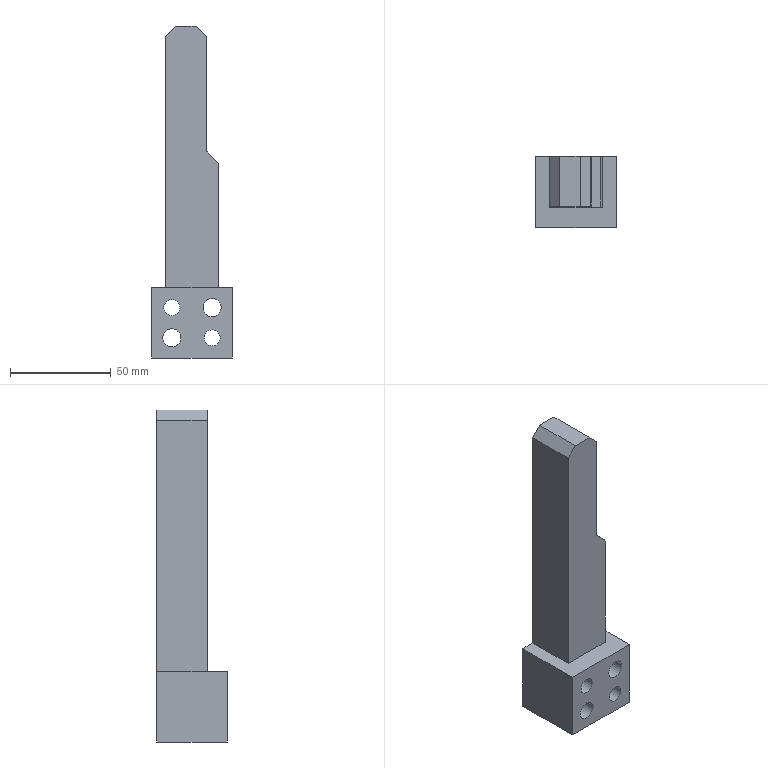Part | STEP file | 车灯-后视镜_id230_x_t | 1 solid | 24 faces | box 40 x 35 x 165 mm | volume 113527 mm3 | plane 16 | cylinder 8 | commonest cylinder face diameters 4 x2 8 x2 9 x2 14 x2
STEP:
#1=CARTESIAN_POINT('',(-100.914,285.,-263.086));
#2=VERTEX_POINT('',#1);
#3=CARTESIAN_POINT('',(-96.086,285.,-267.914));
#4=VERTEX_POINT('',#3);
#5=CARTESIAN_POINT('',(-53.5,285.,-310.5));
#6=DIRECTION('',(0.7071,0.,-0.7071));
#7=VECTOR('',#6,1.);
#8=LINE('',#5,#7);
#9=EDGE_CURVE('',#2,#4,#8,.T.);
#10=ORIENTED_EDGE('',*,*,#9,.T.);
#11=CARTESIAN_POINT('',(-96.086,310.,-267.914));
#12=VERTEX_POINT('',#11);
#13=CARTESIAN_POINT('',(-96.086,310.,-267.914));
#14=DIRECTION('',(0.,1.,0.));
#15=VECTOR('',#14,1.);
#16=LINE('',#13,#15);
#17=EDGE_CURVE('',#4,#12,#16,.T.);
#18=ORIENTED_EDGE('',*,*,#17,.T.);
#19=CARTESIAN_POINT('',(-100.914,310.,-263.086));
#20=VERTEX_POINT('',#19);
#21=CARTESIAN_POINT('',(-53.5,310.,-310.5));
#22=DIRECTION('',(-0.7071,0.,0.7071));
#23=VECTOR('',#22,1.);
#24=LINE('',#21,#23);
#25=EDGE_CURVE('',#12,#20,#24,.T.);
#26=ORIENTED_EDGE('',*,*,#25,.T.);
#27=CARTESIAN_POINT('',(-100.914,285.,-263.086));
#28=DIRECTION('',(0.,-1.,0.));
#29=VECTOR('',#28,1.);
#30=LINE('',#27,#29);
#31=EDGE_CURVE('',#20,#2,#30,.T.);
#32=ORIENTED_EDGE('',*,*,#31,.T.);
#33=EDGE_LOOP('',(#10,#18,#26,#32));
#34=FACE_OUTER_BOUND('',#33,.T.);
#35=CARTESIAN_POINT('',(-95.5,285.,-268.5));
#36=DIRECTION('',(0.7071,0.,0.7071));
#37=DIRECTION('',(-0.7071,0.,0.7071));
#38=AXIS2_PLACEMENT_3D('',#35,#36,#37);
#39=PLANE('',#38);
#40=ADVANCED_FACE('',(#34),#39,.T.);
#41=CARTESIAN_POINT('',(-121.5,285.,-330.5));
#42=VERTEX_POINT('',#41);
#43=CARTESIAN_POINT('',(-121.5,285.,-205.5));
#44=VERTEX_POINT('',#43);
#45=CARTESIAN_POINT('',(-121.5,285.,-365.5));
#46=DIRECTION('',(0.,0.,1.));
#47=VECTOR('',#46,1.);
#48=LINE('',#45,#47);
#49=EDGE_CURVE('',#42,#44,#48,.T.);
#50=ORIENTED_EDGE('',*,*,#49,.T.);
#51=CARTESIAN_POINT('',(-121.5,310.,-205.5));
#52=VERTEX_POINT('',#51);
#53=CARTESIAN_POINT('',(-121.5,310.,-205.5));
#54=DIRECTION('',(0.,1.,0.));
#55=VECTOR('',#54,1.);
#56=LINE('',#53,#55);
#57=EDGE_CURVE('',#44,#52,#56,.T.);
#58=ORIENTED_EDGE('',*,*,#57,.T.);
#59=CARTESIAN_POINT('',(-121.5,310.,-330.5));
#60=VERTEX_POINT('',#59);
#61=CARTESIAN_POINT('',(-121.5,310.,-365.5));
#62=DIRECTION('',(0.,0.,1.));
#63=VECTOR('',#62,1.);
#64=LINE('',#61,#63);
#65=EDGE_CURVE('',#60,#52,#64,.T.);
#66=ORIENTED_EDGE('',*,*,#65,.F.);
#67=CARTESIAN_POINT('',(-121.5,292.5,-330.5));
#68=DIRECTION('',(0.,-1.,0.));
#69=VECTOR('',#68,1.);
#70=LINE('',#67,#69);
#71=EDGE_CURVE('',#60,#42,#70,.T.);
#72=ORIENTED_EDGE('',*,*,#71,.T.);
#73=EDGE_LOOP('',(#50,#58,#66,#72));
#74=FACE_OUTER_BOUND('',#73,.T.);
#75=CARTESIAN_POINT('',(-121.5,292.5,-365.5));
#76=DIRECTION('',(-1.,0.,0.));
#77=DIRECTION('',(0.,0.,-1.));
#78=AXIS2_PLACEMENT_3D('',#75,#76,#77);
#79=PLANE('',#78);
#80=ADVANCED_FACE('',(#74),#79,.T.);
#81=CARTESIAN_POINT('',(-95.5,285.,-330.5));
#82=VERTEX_POINT('',#81);
#83=CARTESIAN_POINT('',(-95.5,285.,-269.328));
#84=VERTEX_POINT('',#83);
#85=CARTESIAN_POINT('',(-95.5,285.,-365.5));
#86=DIRECTION('',(0.,0.,1.));
#87=VECTOR('',#86,1.);
#88=LINE('',#85,#87);
#89=EDGE_CURVE('',#82,#84,#88,.T.);
#90=ORIENTED_EDGE('',*,*,#89,.T.);
#91=CARTESIAN_POINT('',(-97.5,285.,-269.328));
#92=DIRECTION('',(0.,-1.,0.));
#93=DIRECTION('',(0.,0.,1.));
#94=AXIS2_PLACEMENT_3D('',#91,#92,#93);
#95=CIRCLE('',#94,2.);
#96=EDGE_CURVE('',#84,#4,#95,.T.);
#97=ORIENTED_EDGE('',*,*,#96,.T.);
#98=ORIENTED_EDGE('',*,*,#9,.F.);
#99=CARTESIAN_POINT('',(-101.5,285.,-261.672));
#100=VERTEX_POINT('',#99);
#101=CARTESIAN_POINT('',(-99.5,285.,-261.672));
#102=DIRECTION('',(0.,1.,0.));
#103=DIRECTION('',(0.,0.,1.));
#104=AXIS2_PLACEMENT_3D('',#101,#102,#103);
#105=CIRCLE('',#104,2.);
#106=EDGE_CURVE('',#2,#100,#105,.T.);
#107=ORIENTED_EDGE('',*,*,#106,.T.);
#108=CARTESIAN_POINT('',(-101.5,285.,-205.5));
#109=VERTEX_POINT('',#108);
#110=CARTESIAN_POINT('',(-101.5,285.,-365.5));
#111=DIRECTION('',(0.,0.,1.));
#112=VECTOR('',#111,1.);
#113=LINE('',#110,#112);
#114=EDGE_CURVE('',#100,#109,#113,.T.);
#115=ORIENTED_EDGE('',*,*,#114,.T.);
#116=CARTESIAN_POINT('',(-106.5,285.,-200.5));
#117=VERTEX_POINT('',#116);
#118=CARTESIAN_POINT('',(-25.,285.,-282.));
#119=DIRECTION('',(-0.7071,0.,0.7071));
#120=VECTOR('',#119,1.);
#121=LINE('',#118,#120);
#122=EDGE_CURVE('',#109,#117,#121,.T.);
#123=ORIENTED_EDGE('',*,*,#122,.T.);
#124=CARTESIAN_POINT('',(-116.5,285.,-200.5));
#125=VERTEX_POINT('',#124);
#126=CARTESIAN_POINT('',(-108.5,285.,-200.5));
#127=DIRECTION('',(1.,0.,0.));
#128=VECTOR('',#127,1.);
#129=LINE('',#126,#128);
#130=EDGE_CURVE('',#125,#117,#129,.T.);
#131=ORIENTED_EDGE('',*,*,#130,.F.);
#132=CARTESIAN_POINT('',(-195.,285.,-279.));
#133=DIRECTION('',(-0.7071,0.,-0.7071));
#134=VECTOR('',#133,1.);
#135=LINE('',#132,#134);
#136=EDGE_CURVE('',#125,#44,#135,.T.);
#137=ORIENTED_EDGE('',*,*,#136,.T.);
#138=ORIENTED_EDGE('',*,*,#49,.F.);
#139=CARTESIAN_POINT('',(-108.5,285.,-330.5));
#140=DIRECTION('',(1.,0.,0.));
#141=VECTOR('',#140,1.);
#142=LINE('',#139,#141);
#143=EDGE_CURVE('',#42,#82,#142,.T.);
#144=ORIENTED_EDGE('',*,*,#143,.T.);
#145=EDGE_LOOP('',(#90,#97,#98,#107,#115,#123,#131,#137,#138,#144));
#146=FACE_OUTER_BOUND('',#145,.T.);
#147=CARTESIAN_POINT('',(-108.5,285.,-365.5));
#148=DIRECTION('',(0.,-1.,0.));
#149=DIRECTION('',(0.,0.,1.));
#150=AXIS2_PLACEMENT_3D('',#147,#148,#149);
#151=PLANE('',#150);
#152=ADVANCED_FACE('',(#146),#151,.T.);
#153=CARTESIAN_POINT('',(-95.5,310.,-330.5));
#154=VERTEX_POINT('',#153);
#155=CARTESIAN_POINT('',(-95.5,310.,-269.328));
#156=VERTEX_POINT('',#155);
#157=CARTESIAN_POINT('',(-95.5,310.,-365.5));
#158=DIRECTION('',(0.,0.,1.));
#159=VECTOR('',#158,1.);
#160=LINE('',#157,#159);
#161=EDGE_CURVE('',#154,#156,#160,.T.);
#162=ORIENTED_EDGE('',*,*,#161,.T.);
#163=CARTESIAN_POINT('',(-95.5,285.,-269.328));
#164=DIRECTION('',(0.,-1.,0.));
#165=VECTOR('',#164,1.);
#166=LINE('',#163,#165);
#167=EDGE_CURVE('',#156,#84,#166,.T.);
#168=ORIENTED_EDGE('',*,*,#167,.T.);
#169=ORIENTED_EDGE('',*,*,#89,.F.);
#170=CARTESIAN_POINT('',(-95.5,292.5,-330.5));
#171=DIRECTION('',(0.,1.,0.));
#172=VECTOR('',#171,1.);
#173=LINE('',#170,#172);
#174=EDGE_CURVE('',#82,#154,#173,.T.);
#175=ORIENTED_EDGE('',*,*,#174,.T.);
#176=EDGE_LOOP('',(#162,#168,#169,#175));
#177=FACE_OUTER_BOUND('',#176,.T.);
#178=CARTESIAN_POINT('',(-95.5,292.5,-365.5));
#179=DIRECTION('',(1.,0.,0.));
#180=DIRECTION('',(0.,0.,1.));
#181=AXIS2_PLACEMENT_3D('',#178,#179,#180);
#182=PLANE('',#181);
#183=ADVANCED_FACE('',(#177),#182,.T.);
#184=CARTESIAN_POINT('',(-111.5,310.,-355.5));
#185=VERTEX_POINT('',#184);
#186=CARTESIAN_POINT('',(-118.5,310.,-355.5));
#187=DIRECTION('',(0.,-1.,0.));
#188=DIRECTION('',(1.,0.,0.));
#189=AXIS2_PLACEMENT_3D('',#186,#187,#188);
#190=CIRCLE('',#189,7.);
#191=EDGE_CURVE('',#185,#185,#190,.T.);
#192=ORIENTED_EDGE('',*,*,#191,.T.);
#193=EDGE_LOOP('',(#192));
#194=FACE_BOUND('',#193,.T.);
#195=CARTESIAN_POINT('',(-91.5,310.,-340.5));
#196=VERTEX_POINT('',#195);
#197=CARTESIAN_POINT('',(-98.5,310.,-340.5));
#198=DIRECTION('',(0.,-1.,0.));
#199=DIRECTION('',(1.,0.,0.));
#200=AXIS2_PLACEMENT_3D('',#197,#198,#199);
#201=CIRCLE('',#200,7.);
#202=EDGE_CURVE('',#196,#196,#201,.T.);
#203=ORIENTED_EDGE('',*,*,#202,.T.);
#204=EDGE_LOOP('',(#203));
#205=FACE_BOUND('',#204,.T.);
#206=ORIENTED_EDGE('',*,*,#25,.F.);
#207=CARTESIAN_POINT('',(-97.5,310.,-269.328));
#208=DIRECTION('',(0.,1.,0.));
#209=DIRECTION('',(0.,0.,-1.));
#210=AXIS2_PLACEMENT_3D('',#207,#208,#209);
#211=CIRCLE('',#210,2.);
#212=EDGE_CURVE('',#12,#156,#211,.T.);
#213=ORIENTED_EDGE('',*,*,#212,.T.);
#214=ORIENTED_EDGE('',*,*,#161,.F.);
#215=CARTESIAN_POINT('',(-88.5,310.,-330.5));
#216=VERTEX_POINT('',#215);
#217=CARTESIAN_POINT('',(-108.5,310.,-330.5));
#218=DIRECTION('',(-1.,0.,0.));
#219=VECTOR('',#218,1.);
#220=LINE('',#217,#219);
#221=EDGE_CURVE('',#216,#154,#220,.T.);
#222=ORIENTED_EDGE('',*,*,#221,.F.);
#223=CARTESIAN_POINT('',(-88.5,310.,-365.5));
#224=VERTEX_POINT('',#223);
#225=CARTESIAN_POINT('',(-88.5,310.,-365.5));
#226=DIRECTION('',(0.,0.,1.));
#227=VECTOR('',#226,1.);
#228=LINE('',#225,#227);
#229=EDGE_CURVE('',#224,#216,#228,.T.);
#230=ORIENTED_EDGE('',*,*,#229,.F.);
#231=CARTESIAN_POINT('',(-128.5,310.,-365.5));
#232=VERTEX_POINT('',#231);
#233=CARTESIAN_POINT('',(-108.5,310.,-365.5));
#234=DIRECTION('',(-1.,0.,0.));
#235=VECTOR('',#234,1.);
#236=LINE('',#233,#235);
#237=EDGE_CURVE('',#224,#232,#236,.T.);
#238=ORIENTED_EDGE('',*,*,#237,.T.);
#239=CARTESIAN_POINT('',(-128.5,310.,-330.5));
#240=VERTEX_POINT('',#239);
#241=CARTESIAN_POINT('',(-128.5,310.,-365.5));
#242=DIRECTION('',(0.,0.,1.));
#243=VECTOR('',#242,1.);
#244=LINE('',#241,#243);
#245=EDGE_CURVE('',#232,#240,#244,.T.);
#246=ORIENTED_EDGE('',*,*,#245,.T.);
#247=CARTESIAN_POINT('',(-108.5,310.,-330.5));
#248=DIRECTION('',(-1.,0.,0.));
#249=VECTOR('',#248,1.);
#250=LINE('',#247,#249);
#251=EDGE_CURVE('',#60,#240,#250,.T.);
#252=ORIENTED_EDGE('',*,*,#251,.F.);
#253=ORIENTED_EDGE('',*,*,#65,.T.);
#254=CARTESIAN_POINT('',(-116.5,310.,-200.5));
#255=VERTEX_POINT('',#254);
#256=CARTESIAN_POINT('',(-195.,310.,-279.));
#257=DIRECTION('',(0.7071,0.,0.7071));
#258=VECTOR('',#257,1.);
#259=LINE('',#256,#258);
#260=EDGE_CURVE('',#52,#255,#259,.T.);
#261=ORIENTED_EDGE('',*,*,#260,.T.);
#262=CARTESIAN_POINT('',(-106.5,310.,-200.5));
#263=VERTEX_POINT('',#262);
#264=CARTESIAN_POINT('',(-108.5,310.,-200.5));
#265=DIRECTION('',(-1.,0.,0.));
#266=VECTOR('',#265,1.);
#267=LINE('',#264,#266);
#268=EDGE_CURVE('',#263,#255,#267,.T.);
#269=ORIENTED_EDGE('',*,*,#268,.F.);
#270=CARTESIAN_POINT('',(-101.5,310.,-205.5));
#271=VERTEX_POINT('',#270);
#272=CARTESIAN_POINT('',(-25.,310.,-282.));
#273=DIRECTION('',(0.7071,0.,-0.7071));
#274=VECTOR('',#273,1.);
#275=LINE('',#272,#274);
#276=EDGE_CURVE('',#263,#271,#275,.T.);
#277=ORIENTED_EDGE('',*,*,#276,.T.);
#278=CARTESIAN_POINT('',(-101.5,310.,-261.672));
#279=VERTEX_POINT('',#278);
#280=CARTESIAN_POINT('',(-101.5,310.,-365.5));
#281=DIRECTION('',(0.,0.,1.));
#282=VECTOR('',#281,1.);
#283=LINE('',#280,#282);
#284=EDGE_CURVE('',#279,#271,#283,.T.);
#285=ORIENTED_EDGE('',*,*,#284,.F.);
#286=CARTESIAN_POINT('',(-99.5,310.,-261.672));
#287=DIRECTION('',(0.,-1.,0.));
#288=DIRECTION('',(0.,0.,-1.));
#289=AXIS2_PLACEMENT_3D('',#286,#287,#288);
#290=CIRCLE('',#289,2.);
#291=EDGE_CURVE('',#279,#20,#290,.T.);
#292=ORIENTED_EDGE('',*,*,#291,.T.);
#293=EDGE_LOOP('',(#206,#213,#214,#222,#230,#238,#246,#252,#253,#261,#269,#277,#285,#292));
#294=FACE_BOUND('',#293,.T.);
#295=CARTESIAN_POINT('',(-98.5,310.,-359.5));
#296=VERTEX_POINT('',#295);
#297=CARTESIAN_POINT('',(-98.5,310.,-355.5));
#298=DIRECTION('',(0.,-1.,0.));
#299=DIRECTION('',(0.,0.,-1.));
#300=AXIS2_PLACEMENT_3D('',#297,#298,#299);
#301=CIRCLE('',#300,4.);
#302=EDGE_CURVE('',#296,#296,#301,.T.);
#303=ORIENTED_EDGE('',*,*,#302,.T.);
#304=EDGE_LOOP('',(#303));
#305=FACE_BOUND('',#304,.T.);
#306=CARTESIAN_POINT('',(-118.5,310.,-344.5));
#307=VERTEX_POINT('',#306);
#308=CARTESIAN_POINT('',(-118.5,310.,-340.5));
#309=DIRECTION('',(0.,-1.,0.));
#310=DIRECTION('',(0.,0.,-1.));
#311=AXIS2_PLACEMENT_3D('',#308,#309,#310);
#312=CIRCLE('',#311,4.);
#313=EDGE_CURVE('',#307,#307,#312,.T.);
#314=ORIENTED_EDGE('',*,*,#313,.T.);
#315=EDGE_LOOP('',(#314));
#316=FACE_BOUND('',#315,.T.);
#317=CARTESIAN_POINT('',(-108.5,310.,-365.5));
#318=DIRECTION('',(0.,1.,0.));
#319=DIRECTION('',(0.,0.,-1.));
#320=AXIS2_PLACEMENT_3D('',#317,#318,#319);
#321=PLANE('',#320);
#322=ADVANCED_FACE('',(#194,#205,#294,#305,#316),#321,.T.);
#323=CARTESIAN_POINT('',(-88.5,275.,-330.5));
#324=VERTEX_POINT('',#323);
#325=CARTESIAN_POINT('',(-88.5,292.5,-330.5));
#326=DIRECTION('',(0.,1.,0.));
#327=VECTOR('',#326,1.);
#328=LINE('',#325,#327);
#329=EDGE_CURVE('',#324,#216,#328,.T.);
#330=ORIENTED_EDGE('',*,*,#329,.F.);
#331=CARTESIAN_POINT('',(-88.5,275.,-365.5));
#332=VERTEX_POINT('',#331);
#333=CARTESIAN_POINT('',(-88.5,275.,-365.5));
#334=DIRECTION('',(0.,0.,1.));
#335=VECTOR('',#334,1.);
#336=LINE('',#333,#335);
#337=EDGE_CURVE('',#332,#324,#336,.T.);
#338=ORIENTED_EDGE('',*,*,#337,.F.);
#339=CARTESIAN_POINT('',(-88.5,292.5,-365.5));
#340=DIRECTION('',(0.,1.,0.));
#341=VECTOR('',#340,1.);
#342=LINE('',#339,#341);
#343=EDGE_CURVE('',#332,#224,#342,.T.);
#344=ORIENTED_EDGE('',*,*,#343,.T.);
#345=ORIENTED_EDGE('',*,*,#229,.T.);
#346=EDGE_LOOP('',(#330,#338,#344,#345));
#347=FACE_OUTER_BOUND('',#346,.T.);
#348=CARTESIAN_POINT('',(-88.5,292.5,-365.5));
#349=DIRECTION('',(1.,0.,0.));
#350=DIRECTION('',(0.,0.,1.));
#351=AXIS2_PLACEMENT_3D('',#348,#349,#350);
#352=PLANE('',#351);
#353=ADVANCED_FACE('',(#347),#352,.T.);
#354=CARTESIAN_POINT('',(-98.5,275.,-351.5));
#355=VERTEX_POINT('',#354);
#356=CARTESIAN_POINT('',(-98.5,275.,-355.5));
#357=DIRECTION('',(0.,-1.,0.));
#358=DIRECTION('',(0.,0.,1.));
#359=AXIS2_PLACEMENT_3D('',#356,#357,#358);
#360=CIRCLE('',#359,4.);
#361=EDGE_CURVE('',#355,#355,#360,.T.);
#362=ORIENTED_EDGE('',*,*,#361,.F.);
#363=EDGE_LOOP('',(#362));
#364=FACE_BOUND('',#363,.T.);
#365=CARTESIAN_POINT('',(-118.5,275.,-351.));
#366=VERTEX_POINT('',#365);
#367=CARTESIAN_POINT('',(-118.5,275.,-355.5));
#368=DIRECTION('',(0.,-1.,0.));
#369=DIRECTION('',(0.,0.,1.));
#370=AXIS2_PLACEMENT_3D('',#367,#368,#369);
#371=CIRCLE('',#370,4.5);
#372=EDGE_CURVE('',#366,#366,#371,.T.);
#373=ORIENTED_EDGE('',*,*,#372,.F.);
#374=EDGE_LOOP('',(#373));
#375=FACE_BOUND('',#374,.T.);
#376=CARTESIAN_POINT('',(-118.5,275.,-336.5));
#377=VERTEX_POINT('',#376);
#378=CARTESIAN_POINT('',(-118.5,275.,-340.5));
#379=DIRECTION('',(0.,-1.,0.));
#380=DIRECTION('',(0.,0.,1.));
#381=AXIS2_PLACEMENT_3D('',#378,#379,#380);
#382=CIRCLE('',#381,4.);
#383=EDGE_CURVE('',#377,#377,#382,.T.);
#384=ORIENTED_EDGE('',*,*,#383,.F.);
#385=EDGE_LOOP('',(#384));
#386=FACE_BOUND('',#385,.T.);
#387=CARTESIAN_POINT('',(-98.5,275.,-336.));
#388=VERTEX_POINT('',#387);
#389=CARTESIAN_POINT('',(-98.5,275.,-340.5));
#390=DIRECTION('',(0.,-1.,0.));
#391=DIRECTION('',(0.,0.,1.));
#392=AXIS2_PLACEMENT_3D('',#389,#390,#391);
#393=CIRCLE('',#392,4.5);
#394=EDGE_CURVE('',#388,#388,#393,.T.);
#395=ORIENTED_EDGE('',*,*,#394,.F.);
#396=EDGE_LOOP('',(#395));
#397=FACE_BOUND('',#396,.T.);
#398=CARTESIAN_POINT('',(-128.5,275.,-330.5));
#399=VERTEX_POINT('',#398);
#400=CARTESIAN_POINT('',(-108.5,275.,-330.5));
#401=DIRECTION('',(1.,0.,0.));
#402=VECTOR('',#401,1.);
#403=LINE('',#400,#402);
#404=EDGE_CURVE('',#399,#324,#403,.T.);
#405=ORIENTED_EDGE('',*,*,#404,.F.);
#406=CARTESIAN_POINT('',(-128.5,275.,-365.5));
#407=VERTEX_POINT('',#406);
#408=CARTESIAN_POINT('',(-128.5,275.,-365.5));
#409=DIRECTION('',(0.,0.,1.));
#410=VECTOR('',#409,1.);
#411=LINE('',#408,#410);
#412=EDGE_CURVE('',#407,#399,#411,.T.);
#413=ORIENTED_EDGE('',*,*,#412,.F.);
#414=CARTESIAN_POINT('',(-108.5,275.,-365.5));
#415=DIRECTION('',(1.,0.,0.));
#416=VECTOR('',#415,1.);
#417=LINE('',#414,#416);
#418=EDGE_CURVE('',#407,#332,#417,.T.);
#419=ORIENTED_EDGE('',*,*,#418,.T.);
#420=ORIENTED_EDGE('',*,*,#337,.T.);
#421=EDGE_LOOP('',(#405,#413,#419,#420));
#422=FACE_BOUND('',#421,.T.);
#423=CARTESIAN_POINT('',(-108.5,275.,-365.5));
#424=DIRECTION('',(0.,-1.,0.));
#425=DIRECTION('',(0.,0.,1.));
#426=AXIS2_PLACEMENT_3D('',#423,#424,#425);
#427=PLANE('',#426);
#428=ADVANCED_FACE('',(#364,#375,#386,#397,#422),#427,.T.);
#429=CARTESIAN_POINT('',(-128.5,292.5,-365.5));
#430=DIRECTION('',(0.,-1.,0.));
#431=VECTOR('',#430,1.);
#432=LINE('',#429,#431);
#433=EDGE_CURVE('',#232,#407,#432,.T.);
#434=ORIENTED_EDGE('',*,*,#433,.F.);
#435=ORIENTED_EDGE('',*,*,#237,.F.);
#436=ORIENTED_EDGE('',*,*,#343,.F.);
#437=ORIENTED_EDGE('',*,*,#418,.F.);
#438=EDGE_LOOP('',(#434,#435,#436,#437));
#439=FACE_OUTER_BOUND('',#438,.T.);
#440=CARTESIAN_POINT('',(-108.5,292.5,-365.5));
#441=DIRECTION('',(0.,0.,-1.));
#442=DIRECTION('',(1.,0.,0.));
#443=AXIS2_PLACEMENT_3D('',#440,#441,#442);
#444=PLANE('',#443);
#445=ADVANCED_FACE('',(#439),#444,.T.);
#446=CARTESIAN_POINT('',(-128.5,292.5,-330.5));
#447=DIRECTION('',(0.,-1.,0.));
#448=VECTOR('',#447,1.);
#449=LINE('',#446,#448);
#450=EDGE_CURVE('',#240,#399,#449,.T.);
#451=ORIENTED_EDGE('',*,*,#450,.F.);
#452=ORIENTED_EDGE('',*,*,#245,.F.);
#453=ORIENTED_EDGE('',*,*,#433,.T.);
#454=ORIENTED_EDGE('',*,*,#412,.T.);
#455=EDGE_LOOP('',(#451,#452,#453,#454));
#456=FACE_OUTER_BOUND('',#455,.T.);
#457=CARTESIAN_POINT('',(-128.5,292.5,-365.5));
#458=DIRECTION('',(-1.,0.,0.));
#459=DIRECTION('',(0.,0.,-1.));
#460=AXIS2_PLACEMENT_3D('',#457,#458,#459);
#461=PLANE('',#460);
#462=ADVANCED_FACE('',(#456),#461,.T.);
#463=ORIENTED_EDGE('',*,*,#174,.F.);
#464=ORIENTED_EDGE('',*,*,#143,.F.);
#465=ORIENTED_EDGE('',*,*,#71,.F.);
#466=ORIENTED_EDGE('',*,*,#251,.T.);
#467=ORIENTED_EDGE('',*,*,#450,.T.);
#468=ORIENTED_EDGE('',*,*,#404,.T.);
#469=ORIENTED_EDGE('',*,*,#329,.T.);
#470=ORIENTED_EDGE('',*,*,#221,.T.);
#471=EDGE_LOOP('',(#463,#464,#465,#466,#467,#468,#469,#470));
#472=FACE_OUTER_BOUND('',#471,.T.);
#473=CARTESIAN_POINT('',(-108.5,292.5,-330.5));
#474=DIRECTION('',(0.,0.,-1.));
#475=DIRECTION('',(1.,0.,0.));
#476=AXIS2_PLACEMENT_3D('',#473,#474,#475);
#477=PLANE('',#476);
#478=ADVANCED_FACE('',(#472),#477,.F.);
#479=CARTESIAN_POINT('',(-98.5,301.,-336.));
#480=VERTEX_POINT('',#479);
#481=CARTESIAN_POINT('',(-98.5,301.,-340.5));
#482=DIRECTION('',(0.,1.,0.));
#483=DIRECTION('',(0.,0.,1.));
#484=AXIS2_PLACEMENT_3D('',#481,#482,#483);
#485=CIRCLE('',#484,4.5);
#486=EDGE_CURVE('',#480,#480,#485,.T.);
#487=ORIENTED_EDGE('',*,*,#486,.T.);
#488=EDGE_LOOP('',(#487));
#489=FACE_BOUND('',#488,.T.);
#490=ORIENTED_EDGE('',*,*,#394,.T.);
#491=EDGE_LOOP('',(#490));
#492=FACE_BOUND('',#491,.T.);
#493=CARTESIAN_POINT('',(-98.5,310.,-340.5));
#494=DIRECTION('',(0.,-1.,0.));
#495=DIRECTION('',(0.,0.,1.));
#496=AXIS2_PLACEMENT_3D('',#493,#494,#495);
#497=CYLINDRICAL_SURFACE('',#496,4.5);
#498=ADVANCED_FACE('',(#489,#492),#497,.F.);
#499=ORIENTED_EDGE('',*,*,#383,.T.);
#500=EDGE_LOOP('',(#499));
#501=FACE_BOUND('',#500,.T.);
#502=ORIENTED_EDGE('',*,*,#313,.F.);
#503=EDGE_LOOP('',(#502));
#504=FACE_BOUND('',#503,.T.);
#505=CARTESIAN_POINT('',(-118.5,310.,-340.5));
#506=DIRECTION('',(0.,-1.,0.));
#507=DIRECTION('',(0.,0.,1.));
#508=AXIS2_PLACEMENT_3D('',#505,#506,#507);
#509=CYLINDRICAL_SURFACE('',#508,4.);
#510=ADVANCED_FACE('',(#501,#504),#509,.F.);
#511=CARTESIAN_POINT('',(-118.5,301.,-351.));
#512=VERTEX_POINT('',#511);
#513=CARTESIAN_POINT('',(-118.5,301.,-355.5));
#514=DIRECTION('',(0.,1.,0.));
#515=DIRECTION('',(0.,0.,1.));
#516=AXIS2_PLACEMENT_3D('',#513,#514,#515);
#517=CIRCLE('',#516,4.5);
#518=EDGE_CURVE('',#512,#512,#517,.T.);
#519=ORIENTED_EDGE('',*,*,#518,.T.);
#520=EDGE_LOOP('',(#519));
#521=FACE_BOUND('',#520,.T.);
#522=ORIENTED_EDGE('',*,*,#372,.T.);
#523=EDGE_LOOP('',(#522));
#524=FACE_BOUND('',#523,.T.);
#525=CARTESIAN_POINT('',(-118.5,310.,-355.5));
#526=DIRECTION('',(0.,-1.,0.));
#527=DIRECTION('',(0.,0.,1.));
#528=AXIS2_PLACEMENT_3D('',#525,#526,#527);
#529=CYLINDRICAL_SURFACE('',#528,4.5);
#530=ADVANCED_FACE('',(#521,#524),#529,.F.);
#531=ORIENTED_EDGE('',*,*,#361,.T.);
#532=EDGE_LOOP('',(#531));
#533=FACE_BOUND('',#532,.T.);
#534=ORIENTED_EDGE('',*,*,#302,.F.);
#535=EDGE_LOOP('',(#534));
#536=FACE_BOUND('',#535,.T.);
#537=CARTESIAN_POINT('',(-98.5,310.,-355.5));
#538=DIRECTION('',(0.,-1.,0.));
#539=DIRECTION('',(0.,0.,1.));
#540=AXIS2_PLACEMENT_3D('',#537,#538,#539);
#541=CYLINDRICAL_SURFACE('',#540,4.);
#542=ADVANCED_FACE('',(#533,#536),#541,.F.);
#543=ORIENTED_EDGE('',*,*,#130,.T.);
#544=CARTESIAN_POINT('',(-106.5,310.,-200.5));
#545=DIRECTION('',(0.,1.,0.));
#546=VECTOR('',#545,1.);
#547=LINE('',#544,#546);
#548=EDGE_CURVE('',#117,#263,#547,.T.);
#549=ORIENTED_EDGE('',*,*,#548,.T.);
#550=ORIENTED_EDGE('',*,*,#268,.T.);
#551=CARTESIAN_POINT('',(-116.5,285.,-200.5));
#552=DIRECTION('',(0.,-1.,0.));
#553=VECTOR('',#552,1.);
#554=LINE('',#551,#553);
#555=EDGE_CURVE('',#255,#125,#554,.T.);
#556=ORIENTED_EDGE('',*,*,#555,.T.);
#557=EDGE_LOOP('',(#543,#549,#550,#556));
#558=FACE_OUTER_BOUND('',#557,.T.);
#559=CARTESIAN_POINT('',(-121.5,310.,-200.5));
#560=DIRECTION('',(0.,0.,-1.));
#561=DIRECTION('',(1.,0.,0.));
#562=AXIS2_PLACEMENT_3D('',#559,#560,#561);
#563=PLANE('',#562);
#564=ADVANCED_FACE('',(#558),#563,.F.);
#565=ORIENTED_EDGE('',*,*,#114,.F.);
#566=CARTESIAN_POINT('',(-101.5,292.5,-261.672));
#567=DIRECTION('',(0.,1.,0.));
#568=VECTOR('',#567,1.);
#569=LINE('',#566,#568);
#570=EDGE_CURVE('',#100,#279,#569,.T.);
#571=ORIENTED_EDGE('',*,*,#570,.T.);
#572=ORIENTED_EDGE('',*,*,#284,.T.);
#573=CARTESIAN_POINT('',(-101.5,285.,-205.5));
#574=DIRECTION('',(0.,-1.,0.));
#575=VECTOR('',#574,1.);
#576=LINE('',#573,#575);
#577=EDGE_CURVE('',#271,#109,#576,.T.);
#578=ORIENTED_EDGE('',*,*,#577,.T.);
#579=EDGE_LOOP('',(#565,#571,#572,#578));
#580=FACE_OUTER_BOUND('',#579,.T.);
#581=CARTESIAN_POINT('',(-101.5,292.5,-365.5));
#582=DIRECTION('',(1.,0.,0.));
#583=DIRECTION('',(0.,0.,1.));
#584=AXIS2_PLACEMENT_3D('',#581,#582,#583);
#585=PLANE('',#584);
#586=ADVANCED_FACE('',(#580),#585,.T.);
#587=ORIENTED_EDGE('',*,*,#122,.F.);
#588=ORIENTED_EDGE('',*,*,#577,.F.);
#589=ORIENTED_EDGE('',*,*,#276,.F.);
#590=ORIENTED_EDGE('',*,*,#548,.F.);
#591=EDGE_LOOP('',(#587,#588,#589,#590));
#592=FACE_OUTER_BOUND('',#591,.T.);
#593=CARTESIAN_POINT('',(-106.5,310.,-200.5));
#594=DIRECTION('',(0.7071,0.,0.7071));
#595=DIRECTION('',(-0.7071,0.,0.7071));
#596=AXIS2_PLACEMENT_3D('',#593,#594,#595);
#597=PLANE('',#596);
#598=ADVANCED_FACE('',(#592),#597,.T.);
#599=ORIENTED_EDGE('',*,*,#260,.F.);
#600=ORIENTED_EDGE('',*,*,#57,.F.);
#601=ORIENTED_EDGE('',*,*,#136,.F.);
#602=ORIENTED_EDGE('',*,*,#555,.F.);
#603=EDGE_LOOP('',(#599,#600,#601,#602));
#604=FACE_OUTER_BOUND('',#603,.T.);
#605=CARTESIAN_POINT('',(-116.5,310.,-200.5));
#606=DIRECTION('',(-0.7071,0.,0.7071));
#607=DIRECTION('',(-0.7071,0.,-0.7071));
#608=AXIS2_PLACEMENT_3D('',#605,#606,#607);
#609=PLANE('',#608);
#610=ADVANCED_FACE('',(#604),#609,.T.);
#611=ORIENTED_EDGE('',*,*,#96,.F.);
#612=ORIENTED_EDGE('',*,*,#167,.F.);
#613=ORIENTED_EDGE('',*,*,#212,.F.);
#614=ORIENTED_EDGE('',*,*,#17,.F.);
#615=EDGE_LOOP('',(#611,#612,#613,#614));
#616=FACE_OUTER_BOUND('',#615,.T.);
#617=CARTESIAN_POINT('',(-97.5,285.,-269.328));
#618=DIRECTION('',(0.,1.,0.));
#619=DIRECTION('',(0.,0.,-1.));
#620=AXIS2_PLACEMENT_3D('',#617,#618,#619);
#621=CYLINDRICAL_SURFACE('',#620,2.);
#622=ADVANCED_FACE('',(#616),#621,.T.);
#623=ORIENTED_EDGE('',*,*,#106,.F.);
#624=ORIENTED_EDGE('',*,*,#31,.F.);
#625=ORIENTED_EDGE('',*,*,#291,.F.);
#626=ORIENTED_EDGE('',*,*,#570,.F.);
#627=EDGE_LOOP('',(#623,#624,#625,#626));
#628=FACE_OUTER_BOUND('',#627,.T.);
#629=CARTESIAN_POINT('',(-99.5,292.5,-261.672));
#630=DIRECTION('',(0.,-1.,0.));
#631=DIRECTION('',(0.,0.,1.));
#632=AXIS2_PLACEMENT_3D('',#629,#630,#631);
#633=CYLINDRICAL_SURFACE('',#632,2.);
#634=ADVANCED_FACE('',(#628),#633,.F.);
#635=ORIENTED_EDGE('',*,*,#486,.F.);
#636=EDGE_LOOP('',(#635));
#637=FACE_BOUND('',#636,.T.);
#638=CARTESIAN_POINT('',(-105.5,301.,-340.5));
#639=VERTEX_POINT('',#638);
#640=CARTESIAN_POINT('',(-98.5,301.,-340.5));
#641=DIRECTION('',(0.,1.,0.));
#642=DIRECTION('',(-1.,0.,0.));
#643=AXIS2_PLACEMENT_3D('',#640,#641,#642);
#644=CIRCLE('',#643,7.);
#645=EDGE_CURVE('',#639,#639,#644,.T.);
#646=ORIENTED_EDGE('',*,*,#645,.T.);
#647=EDGE_LOOP('',(#646));
#648=FACE_BOUND('',#647,.T.);
#649=CARTESIAN_POINT('',(-98.5,301.,-340.5));
#650=DIRECTION('',(0.,-1.,0.));
#651=DIRECTION('',(1.,0.,0.));
#652=AXIS2_PLACEMENT_3D('',#649,#650,#651);
#653=PLANE('',#652);
#654=ADVANCED_FACE('',(#637,#648),#653,.F.);
#655=ORIENTED_EDGE('',*,*,#645,.F.);
#656=EDGE_LOOP('',(#655));
#657=FACE_BOUND('',#656,.T.);
#658=ORIENTED_EDGE('',*,*,#202,.F.);
#659=EDGE_LOOP('',(#658));
#660=FACE_BOUND('',#659,.T.);
#661=CARTESIAN_POINT('',(-98.5,310.,-340.5));
#662=DIRECTION('',(0.,-1.,0.));
#663=DIRECTION('',(1.,0.,0.));
#664=AXIS2_PLACEMENT_3D('',#661,#662,#663);
#665=CYLINDRICAL_SURFACE('',#664,7.);
#666=ADVANCED_FACE('',(#657,#660),#665,.F.);
#667=ORIENTED_EDGE('',*,*,#518,.F.);
#668=EDGE_LOOP('',(#667));
#669=FACE_BOUND('',#668,.T.);
#670=CARTESIAN_POINT('',(-125.5,301.,-355.5));
#671=VERTEX_POINT('',#670);
#672=CARTESIAN_POINT('',(-118.5,301.,-355.5));
#673=DIRECTION('',(0.,1.,0.));
#674=DIRECTION('',(-1.,0.,0.));
#675=AXIS2_PLACEMENT_3D('',#672,#673,#674);
#676=CIRCLE('',#675,7.);
#677=EDGE_CURVE('',#671,#671,#676,.T.);
#678=ORIENTED_EDGE('',*,*,#677,.T.);
#679=EDGE_LOOP('',(#678));
#680=FACE_BOUND('',#679,.T.);
#681=CARTESIAN_POINT('',(-118.5,301.,-355.5));
#682=DIRECTION('',(0.,-1.,0.));
#683=DIRECTION('',(1.,0.,0.));
#684=AXIS2_PLACEMENT_3D('',#681,#682,#683);
#685=PLANE('',#684);
#686=ADVANCED_FACE('',(#669,#680),#685,.F.);
#687=ORIENTED_EDGE('',*,*,#677,.F.);
#688=EDGE_LOOP('',(#687));
#689=FACE_BOUND('',#688,.T.);
#690=ORIENTED_EDGE('',*,*,#191,.F.);
#691=EDGE_LOOP('',(#690));
#692=FACE_BOUND('',#691,.T.);
#693=CARTESIAN_POINT('',(-118.5,310.,-355.5));
#694=DIRECTION('',(0.,-1.,0.));
#695=DIRECTION('',(1.,0.,0.));
#696=AXIS2_PLACEMENT_3D('',#693,#694,#695);
#697=CYLINDRICAL_SURFACE('',#696,7.);
#698=ADVANCED_FACE('',(#689,#692),#697,.F.);
#699=CLOSED_SHELL('',(#40,#80,#152,#183,#322,#353,#428,#445,#462,#478,#498,#510,#530,#542,#564,#586,#598,#610,#622,#634,#654,#666,#686,#698));
#700=MANIFOLD_SOLID_BREP('',#699);
#701=(LENGTH_UNIT()NAMED_UNIT(*)SI_UNIT(.MILLI.,.METRE.));
#702=UNCERTAINTY_MEASURE_WITH_UNIT(LENGTH_MEASURE(0.00002),#701,'','');
#703=(NAMED_UNIT(*)PLANE_ANGLE_UNIT()SI_UNIT($,.RADIAN.));
#704=PLANE_ANGLE_MEASURE_WITH_UNIT(PLANE_ANGLE_MEASURE(0.01745),#703);
#705=DIMENSIONAL_EXPONENTS(0.,0.,0.,0.,0.,0.,0.);
#706=(CONVERSION_BASED_UNIT('DEGREE',#704)NAMED_UNIT(#705)PLANE_ANGLE_UNIT());
#707=(NAMED_UNIT(*)SI_UNIT($,.STERADIAN.)SOLID_ANGLE_UNIT());
#708=(GEOMETRIC_REPRESENTATION_CONTEXT(3)GLOBAL_UNCERTAINTY_ASSIGNED_CONTEXT((#702))GLOBAL_UNIT_ASSIGNED_CONTEXT((#701,#706,#707))REPRESENTATION_CONTEXT('',''));
#709=ADVANCED_BREP_SHAPE_REPRESENTATION('',(#700),#708);